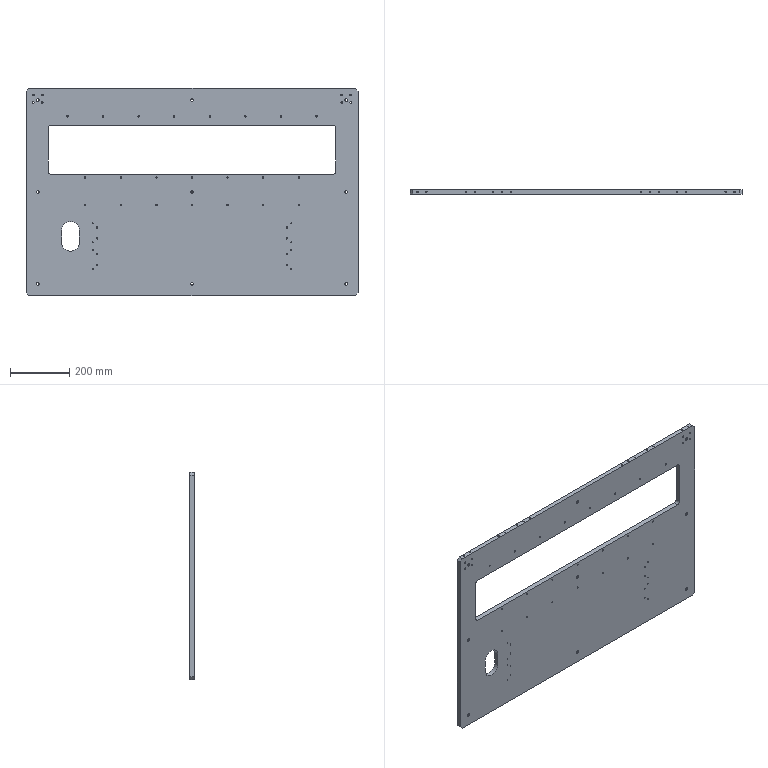Part | SolidWorks | features HoleWzd 10, Cut 2, Chamfer 1, Extrusion 1, Fillet 1 | 1 solid | 216 faces | box 1120 x 15 x 700 mm | volume 9247441 mm3 | cylinder 163 | cone 28 | plane 25 | commonest cylinder face diameters 4.2 x64 5 x40 9 x18 15 x18 3.3 x16 20 x4